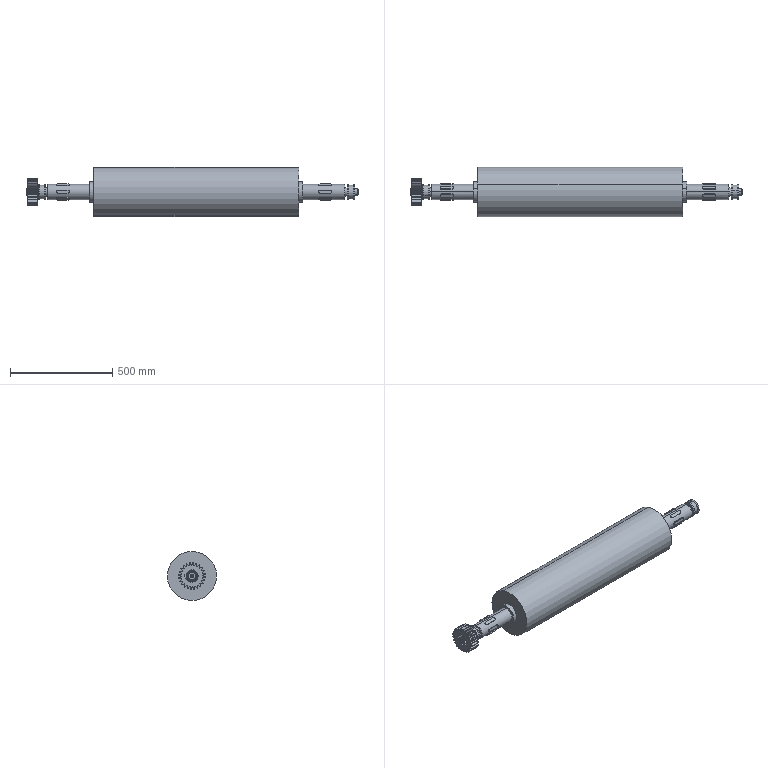Part | SolidWorks | 82 solids | 1230 faces | box 1620 x 240 x 240 mm | volume 47963856 mm3 | cylinder 541 | spline 372 | plane 277 | cone 40 | commonest cylinder face diameters 41.25 x132 43.75 x132 15 x70 48 x52 107.498 x25 130 x24